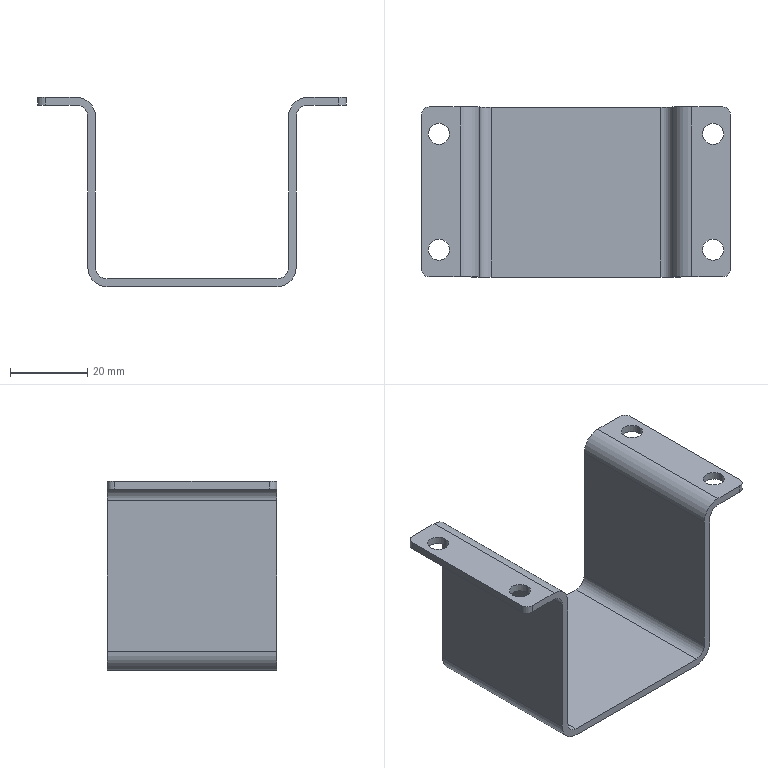Part | STEP file | Air switch blank | 1 solid | 34 faces | box 80 x 44 x 49 mm | volume 14511 mm3 | cylinder 20 | plane 14 | commonest cylinder face diameters 5.5 x8 4 x4 6 x4 10 x4